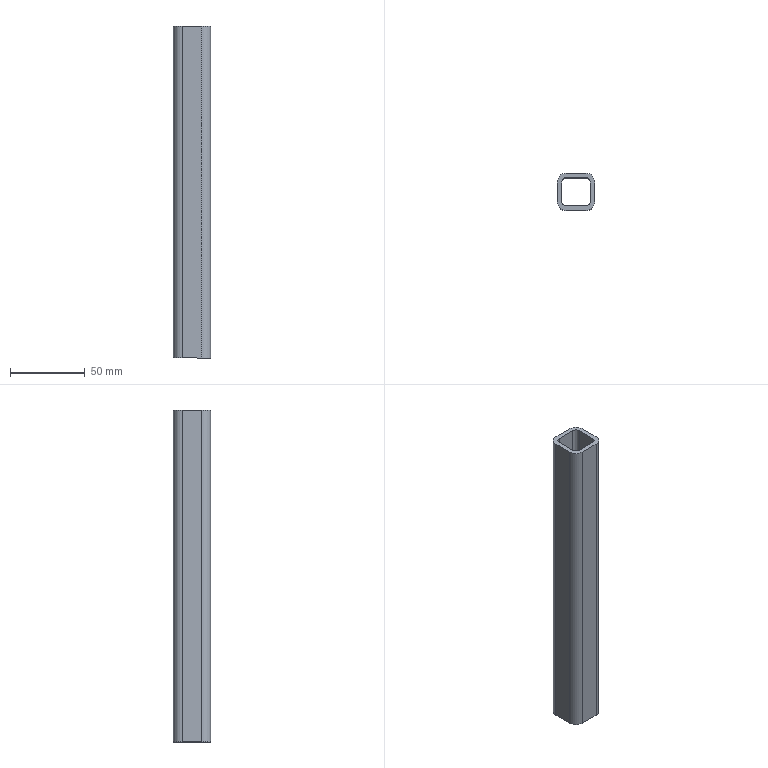Part | STEP file | ISO 10799-2 25x25x3 1784905468899 | 1 solid | 18 faces | box 25 x 25 x 222.2 mm | volume 53511 mm3 | plane 10 | cylinder 8 | commonest cylinder face diameters 6 x4 12 x4
STEP:
#1=CARTESIAN_POINT('',(-6.5,-9.5,247.2));
#2=VERTEX_POINT('',#1);
#3=CARTESIAN_POINT('',(6.5,-9.5,247.2));
#4=VERTEX_POINT('',#3);
#5=CARTESIAN_POINT('',(3.25,-9.5,247.2));
#6=DIRECTION('',(1.,0.,0.));
#7=VECTOR('',#6,10.);
#8=LINE('',#5,#7);
#9=EDGE_CURVE('',#2,#4,#8,.T.);
#10=ORIENTED_EDGE('',*,*,#9,.T.);
#11=CARTESIAN_POINT('',(6.5,-9.5,25.));
#12=VERTEX_POINT('',#11);
#13=CARTESIAN_POINT('',(6.5,-9.5,0.));
#14=DIRECTION('',(0.,0.,1.));
#15=VECTOR('',#14,10.);
#16=LINE('',#13,#15);
#17=EDGE_CURVE('',#12,#4,#16,.T.);
#18=ORIENTED_EDGE('',*,*,#17,.F.);
#19=CARTESIAN_POINT('',(-6.5,-9.5,25.));
#20=VERTEX_POINT('',#19);
#21=CARTESIAN_POINT('',(3.25,-9.5,25.));
#22=DIRECTION('',(1.,0.,0.));
#23=VECTOR('',#22,10.);
#24=LINE('',#21,#23);
#25=EDGE_CURVE('',#20,#12,#24,.T.);
#26=ORIENTED_EDGE('',*,*,#25,.F.);
#27=CARTESIAN_POINT('',(-6.5,-9.5,0.));
#28=DIRECTION('',(0.,0.,1.));
#29=VECTOR('',#28,10.);
#30=LINE('',#27,#29);
#31=EDGE_CURVE('',#20,#2,#30,.T.);
#32=ORIENTED_EDGE('',*,*,#31,.T.);
#33=EDGE_LOOP('',(#10,#18,#26,#32));
#34=FACE_OUTER_BOUND('',#33,.T.);
#35=CARTESIAN_POINT('',(6.5,-9.5,0.));
#36=DIRECTION('',(0.,-1.,0.));
#37=DIRECTION('',(0.,0.,-1.));
#38=AXIS2_PLACEMENT_3D('',#35,#36,#37);
#39=PLANE('',#38);
#40=ADVANCED_FACE('',(#34),#39,.F.);
#41=CARTESIAN_POINT('',(9.5,-6.5,247.2));
#42=VERTEX_POINT('',#41);
#43=CARTESIAN_POINT('',(6.5,-6.5,247.2));
#44=DIRECTION('',(0.,0.,1.));
#45=DIRECTION('',(0.,1.,0.));
#46=AXIS2_PLACEMENT_3D('',#43,#44,#45);
#47=CIRCLE('',#46,3.);
#48=EDGE_CURVE('',#4,#42,#47,.T.);
#49=ORIENTED_EDGE('',*,*,#48,.T.);
#50=CARTESIAN_POINT('',(9.5,-6.5,25.));
#51=VERTEX_POINT('',#50);
#52=CARTESIAN_POINT('',(9.5,-6.5,0.));
#53=DIRECTION('',(0.,0.,1.));
#54=VECTOR('',#53,10.);
#55=LINE('',#52,#54);
#56=EDGE_CURVE('',#51,#42,#55,.T.);
#57=ORIENTED_EDGE('',*,*,#56,.F.);
#58=CARTESIAN_POINT('',(6.5,-6.5,25.));
#59=DIRECTION('',(0.,0.,1.));
#60=DIRECTION('',(0.,1.,0.));
#61=AXIS2_PLACEMENT_3D('',#58,#59,#60);
#62=CIRCLE('',#61,3.);
#63=EDGE_CURVE('',#12,#51,#62,.T.);
#64=ORIENTED_EDGE('',*,*,#63,.F.);
#65=ORIENTED_EDGE('',*,*,#17,.T.);
#66=EDGE_LOOP('',(#49,#57,#64,#65));
#67=FACE_OUTER_BOUND('',#66,.T.);
#68=CARTESIAN_POINT('',(6.5,-6.5,0.));
#69=DIRECTION('',(0.,0.,1.));
#70=DIRECTION('',(0.,1.,0.));
#71=AXIS2_PLACEMENT_3D('',#68,#69,#70);
#72=CYLINDRICAL_SURFACE('',#71,3.);
#73=ADVANCED_FACE('',(#67),#72,.F.);
#74=CARTESIAN_POINT('',(9.5,6.5,247.2));
#75=VERTEX_POINT('',#74);
#76=CARTESIAN_POINT('',(9.5,3.25,247.2));
#77=DIRECTION('',(0.,1.,0.));
#78=VECTOR('',#77,10.);
#79=LINE('',#76,#78);
#80=EDGE_CURVE('',#42,#75,#79,.T.);
#81=ORIENTED_EDGE('',*,*,#80,.T.);
#82=CARTESIAN_POINT('',(9.5,6.5,25.));
#83=VERTEX_POINT('',#82);
#84=CARTESIAN_POINT('',(9.5,6.5,0.));
#85=DIRECTION('',(0.,0.,1.));
#86=VECTOR('',#85,10.);
#87=LINE('',#84,#86);
#88=EDGE_CURVE('',#83,#75,#87,.T.);
#89=ORIENTED_EDGE('',*,*,#88,.F.);
#90=CARTESIAN_POINT('',(9.5,3.25,25.));
#91=DIRECTION('',(0.,1.,0.));
#92=VECTOR('',#91,10.);
#93=LINE('',#90,#92);
#94=EDGE_CURVE('',#51,#83,#93,.T.);
#95=ORIENTED_EDGE('',*,*,#94,.F.);
#96=ORIENTED_EDGE('',*,*,#56,.T.);
#97=EDGE_LOOP('',(#81,#89,#95,#96));
#98=FACE_OUTER_BOUND('',#97,.T.);
#99=CARTESIAN_POINT('',(9.5,6.5,0.));
#100=DIRECTION('',(1.,0.,0.));
#101=DIRECTION('',(0.,0.,-1.));
#102=AXIS2_PLACEMENT_3D('',#99,#100,#101);
#103=PLANE('',#102);
#104=ADVANCED_FACE('',(#98),#103,.F.);
#105=CARTESIAN_POINT('',(6.5,9.5,247.2));
#106=VERTEX_POINT('',#105);
#107=CARTESIAN_POINT('',(6.5,6.5,247.2));
#108=DIRECTION('',(0.,0.,1.));
#109=DIRECTION('',(-1.,0.,0.));
#110=AXIS2_PLACEMENT_3D('',#107,#108,#109);
#111=CIRCLE('',#110,3.);
#112=EDGE_CURVE('',#75,#106,#111,.T.);
#113=ORIENTED_EDGE('',*,*,#112,.T.);
#114=CARTESIAN_POINT('',(6.5,9.5,25.));
#115=VERTEX_POINT('',#114);
#116=CARTESIAN_POINT('',(6.5,9.5,0.));
#117=DIRECTION('',(0.,0.,1.));
#118=VECTOR('',#117,10.);
#119=LINE('',#116,#118);
#120=EDGE_CURVE('',#115,#106,#119,.T.);
#121=ORIENTED_EDGE('',*,*,#120,.F.);
#122=CARTESIAN_POINT('',(6.5,6.5,25.));
#123=DIRECTION('',(0.,0.,1.));
#124=DIRECTION('',(-1.,0.,0.));
#125=AXIS2_PLACEMENT_3D('',#122,#123,#124);
#126=CIRCLE('',#125,3.);
#127=EDGE_CURVE('',#83,#115,#126,.T.);
#128=ORIENTED_EDGE('',*,*,#127,.F.);
#129=ORIENTED_EDGE('',*,*,#88,.T.);
#130=EDGE_LOOP('',(#113,#121,#128,#129));
#131=FACE_OUTER_BOUND('',#130,.T.);
#132=CARTESIAN_POINT('',(6.5,6.5,0.));
#133=DIRECTION('',(0.,0.,1.));
#134=DIRECTION('',(-1.,0.,0.));
#135=AXIS2_PLACEMENT_3D('',#132,#133,#134);
#136=CYLINDRICAL_SURFACE('',#135,3.);
#137=ADVANCED_FACE('',(#131),#136,.F.);
#138=CARTESIAN_POINT('',(12.5,6.5,247.2));
#139=VERTEX_POINT('',#138);
#140=CARTESIAN_POINT('',(12.5,-6.5,247.2));
#141=VERTEX_POINT('',#140);
#142=CARTESIAN_POINT('',(12.5,3.25,247.2));
#143=DIRECTION('',(0.,-1.,0.));
#144=VECTOR('',#143,10.);
#145=LINE('',#142,#144);
#146=EDGE_CURVE('',#139,#141,#145,.T.);
#147=ORIENTED_EDGE('',*,*,#146,.T.);
#148=CARTESIAN_POINT('',(12.5,-6.5,25.));
#149=VERTEX_POINT('',#148);
#150=CARTESIAN_POINT('',(12.5,-6.5,0.));
#151=DIRECTION('',(0.,0.,1.));
#152=VECTOR('',#151,10.);
#153=LINE('',#150,#152);
#154=EDGE_CURVE('',#149,#141,#153,.T.);
#155=ORIENTED_EDGE('',*,*,#154,.F.);
#156=CARTESIAN_POINT('',(12.5,6.5,25.));
#157=VERTEX_POINT('',#156);
#158=CARTESIAN_POINT('',(12.5,3.25,25.));
#159=DIRECTION('',(0.,-1.,0.));
#160=VECTOR('',#159,10.);
#161=LINE('',#158,#160);
#162=EDGE_CURVE('',#157,#149,#161,.T.);
#163=ORIENTED_EDGE('',*,*,#162,.F.);
#164=CARTESIAN_POINT('',(12.5,6.5,0.));
#165=DIRECTION('',(0.,0.,1.));
#166=VECTOR('',#165,10.);
#167=LINE('',#164,#166);
#168=EDGE_CURVE('',#157,#139,#167,.T.);
#169=ORIENTED_EDGE('',*,*,#168,.T.);
#170=EDGE_LOOP('',(#147,#155,#163,#169));
#171=FACE_OUTER_BOUND('',#170,.T.);
#172=CARTESIAN_POINT('',(12.5,6.5,0.));
#173=DIRECTION('',(1.,0.,0.));
#174=DIRECTION('',(0.,0.,-1.));
#175=AXIS2_PLACEMENT_3D('',#172,#173,#174);
#176=PLANE('',#175);
#177=ADVANCED_FACE('',(#171),#176,.T.);
#178=CARTESIAN_POINT('',(6.5,-12.5,247.2));
#179=VERTEX_POINT('',#178);
#180=CARTESIAN_POINT('',(6.5,-6.5,247.2));
#181=DIRECTION('',(0.,0.,-1.));
#182=DIRECTION('',(0.,1.,0.));
#183=AXIS2_PLACEMENT_3D('',#180,#181,#182);
#184=CIRCLE('',#183,6.);
#185=EDGE_CURVE('',#141,#179,#184,.T.);
#186=ORIENTED_EDGE('',*,*,#185,.T.);
#187=CARTESIAN_POINT('',(6.5,-12.5,25.));
#188=VERTEX_POINT('',#187);
#189=CARTESIAN_POINT('',(6.5,-12.5,0.));
#190=DIRECTION('',(0.,0.,1.));
#191=VECTOR('',#190,10.);
#192=LINE('',#189,#191);
#193=EDGE_CURVE('',#188,#179,#192,.T.);
#194=ORIENTED_EDGE('',*,*,#193,.F.);
#195=CARTESIAN_POINT('',(6.5,-6.5,25.));
#196=DIRECTION('',(0.,0.,-1.));
#197=DIRECTION('',(0.,1.,0.));
#198=AXIS2_PLACEMENT_3D('',#195,#196,#197);
#199=CIRCLE('',#198,6.);
#200=EDGE_CURVE('',#149,#188,#199,.T.);
#201=ORIENTED_EDGE('',*,*,#200,.F.);
#202=ORIENTED_EDGE('',*,*,#154,.T.);
#203=EDGE_LOOP('',(#186,#194,#201,#202));
#204=FACE_OUTER_BOUND('',#203,.T.);
#205=CARTESIAN_POINT('',(6.5,-6.5,0.));
#206=DIRECTION('',(0.,0.,1.));
#207=DIRECTION('',(0.,1.,0.));
#208=AXIS2_PLACEMENT_3D('',#205,#206,#207);
#209=CYLINDRICAL_SURFACE('',#208,6.);
#210=ADVANCED_FACE('',(#204),#209,.T.);
#211=CARTESIAN_POINT('',(-6.5,-12.5,247.2));
#212=VERTEX_POINT('',#211);
#213=CARTESIAN_POINT('',(3.25,-12.5,247.2));
#214=DIRECTION('',(-1.,0.,0.));
#215=VECTOR('',#214,10.);
#216=LINE('',#213,#215);
#217=EDGE_CURVE('',#179,#212,#216,.T.);
#218=ORIENTED_EDGE('',*,*,#217,.T.);
#219=CARTESIAN_POINT('',(-6.5,-12.5,25.));
#220=VERTEX_POINT('',#219);
#221=CARTESIAN_POINT('',(-6.5,-12.5,0.));
#222=DIRECTION('',(0.,0.,1.));
#223=VECTOR('',#222,10.);
#224=LINE('',#221,#223);
#225=EDGE_CURVE('',#220,#212,#224,.T.);
#226=ORIENTED_EDGE('',*,*,#225,.F.);
#227=CARTESIAN_POINT('',(3.25,-12.5,25.));
#228=DIRECTION('',(-1.,0.,0.));
#229=VECTOR('',#228,10.);
#230=LINE('',#227,#229);
#231=EDGE_CURVE('',#188,#220,#230,.T.);
#232=ORIENTED_EDGE('',*,*,#231,.F.);
#233=ORIENTED_EDGE('',*,*,#193,.T.);
#234=EDGE_LOOP('',(#218,#226,#232,#233));
#235=FACE_OUTER_BOUND('',#234,.T.);
#236=CARTESIAN_POINT('',(6.5,-12.5,0.));
#237=DIRECTION('',(0.,-1.,0.));
#238=DIRECTION('',(0.,0.,-1.));
#239=AXIS2_PLACEMENT_3D('',#236,#237,#238);
#240=PLANE('',#239);
#241=ADVANCED_FACE('',(#235),#240,.T.);
#242=CARTESIAN_POINT('',(-12.5,-6.5,247.2));
#243=VERTEX_POINT('',#242);
#244=CARTESIAN_POINT('',(-6.5,-6.5,247.2));
#245=DIRECTION('',(0.,0.,-1.));
#246=DIRECTION('',(1.,0.,0.));
#247=AXIS2_PLACEMENT_3D('',#244,#245,#246);
#248=CIRCLE('',#247,6.);
#249=EDGE_CURVE('',#212,#243,#248,.T.);
#250=ORIENTED_EDGE('',*,*,#249,.T.);
#251=CARTESIAN_POINT('',(-12.5,-6.5,25.));
#252=VERTEX_POINT('',#251);
#253=CARTESIAN_POINT('',(-12.5,-6.5,0.));
#254=DIRECTION('',(0.,0.,1.));
#255=VECTOR('',#254,10.);
#256=LINE('',#253,#255);
#257=EDGE_CURVE('',#252,#243,#256,.T.);
#258=ORIENTED_EDGE('',*,*,#257,.F.);
#259=CARTESIAN_POINT('',(-6.5,-6.5,25.));
#260=DIRECTION('',(0.,0.,-1.));
#261=DIRECTION('',(1.,0.,0.));
#262=AXIS2_PLACEMENT_3D('',#259,#260,#261);
#263=CIRCLE('',#262,6.);
#264=EDGE_CURVE('',#220,#252,#263,.T.);
#265=ORIENTED_EDGE('',*,*,#264,.F.);
#266=ORIENTED_EDGE('',*,*,#225,.T.);
#267=EDGE_LOOP('',(#250,#258,#265,#266));
#268=FACE_OUTER_BOUND('',#267,.T.);
#269=CARTESIAN_POINT('',(-6.5,-6.5,0.));
#270=DIRECTION('',(0.,0.,1.));
#271=DIRECTION('',(1.,0.,0.));
#272=AXIS2_PLACEMENT_3D('',#269,#270,#271);
#273=CYLINDRICAL_SURFACE('',#272,6.);
#274=ADVANCED_FACE('',(#268),#273,.T.);
#275=CARTESIAN_POINT('',(-6.5,9.5,247.2));
#276=VERTEX_POINT('',#275);
#277=CARTESIAN_POINT('',(-3.25,9.5,247.2));
#278=DIRECTION('',(-1.,0.,0.));
#279=VECTOR('',#278,10.);
#280=LINE('',#277,#279);
#281=EDGE_CURVE('',#106,#276,#280,.T.);
#282=ORIENTED_EDGE('',*,*,#281,.T.);
#283=CARTESIAN_POINT('',(-6.5,9.5,25.));
#284=VERTEX_POINT('',#283);
#285=CARTESIAN_POINT('',(-6.5,9.5,0.));
#286=DIRECTION('',(0.,0.,1.));
#287=VECTOR('',#286,10.);
#288=LINE('',#285,#287);
#289=EDGE_CURVE('',#284,#276,#288,.T.);
#290=ORIENTED_EDGE('',*,*,#289,.F.);
#291=CARTESIAN_POINT('',(-3.25,9.5,25.));
#292=DIRECTION('',(-1.,0.,0.));
#293=VECTOR('',#292,10.);
#294=LINE('',#291,#293);
#295=EDGE_CURVE('',#115,#284,#294,.T.);
#296=ORIENTED_EDGE('',*,*,#295,.F.);
#297=ORIENTED_EDGE('',*,*,#120,.T.);
#298=EDGE_LOOP('',(#282,#290,#296,#297));
#299=FACE_OUTER_BOUND('',#298,.T.);
#300=CARTESIAN_POINT('',(-6.5,9.5,0.));
#301=DIRECTION('',(0.,1.,0.));
#302=DIRECTION('',(0.,0.,1.));
#303=AXIS2_PLACEMENT_3D('',#300,#301,#302);
#304=PLANE('',#303);
#305=ADVANCED_FACE('',(#299),#304,.F.);
#306=CARTESIAN_POINT('',(-9.5,-6.5,247.2));
#307=VERTEX_POINT('',#306);
#308=CARTESIAN_POINT('',(-6.5,-6.5,247.2));
#309=DIRECTION('',(0.,0.,1.));
#310=DIRECTION('',(1.,0.,0.));
#311=AXIS2_PLACEMENT_3D('',#308,#309,#310);
#312=CIRCLE('',#311,3.);
#313=EDGE_CURVE('',#307,#2,#312,.T.);
#314=ORIENTED_EDGE('',*,*,#313,.T.);
#315=ORIENTED_EDGE('',*,*,#31,.F.);
#316=CARTESIAN_POINT('',(-9.5,-6.5,25.));
#317=VERTEX_POINT('',#316);
#318=CARTESIAN_POINT('',(-6.5,-6.5,25.));
#319=DIRECTION('',(0.,0.,1.));
#320=DIRECTION('',(1.,0.,0.));
#321=AXIS2_PLACEMENT_3D('',#318,#319,#320);
#322=CIRCLE('',#321,3.);
#323=EDGE_CURVE('',#317,#20,#322,.T.);
#324=ORIENTED_EDGE('',*,*,#323,.F.);
#325=CARTESIAN_POINT('',(-9.5,-6.5,0.));
#326=DIRECTION('',(0.,0.,1.));
#327=VECTOR('',#326,10.);
#328=LINE('',#325,#327);
#329=EDGE_CURVE('',#317,#307,#328,.T.);
#330=ORIENTED_EDGE('',*,*,#329,.T.);
#331=EDGE_LOOP('',(#314,#315,#324,#330));
#332=FACE_OUTER_BOUND('',#331,.T.);
#333=CARTESIAN_POINT('',(-6.5,-6.5,0.));
#334=DIRECTION('',(0.,0.,1.));
#335=DIRECTION('',(1.,0.,0.));
#336=AXIS2_PLACEMENT_3D('',#333,#334,#335);
#337=CYLINDRICAL_SURFACE('',#336,3.);
#338=ADVANCED_FACE('',(#332),#337,.F.);
#339=CARTESIAN_POINT('',(-9.5,6.5,247.2));
#340=VERTEX_POINT('',#339);
#341=CARTESIAN_POINT('',(-9.5,-3.25,247.2));
#342=DIRECTION('',(0.,-1.,0.));
#343=VECTOR('',#342,10.);
#344=LINE('',#341,#343);
#345=EDGE_CURVE('',#340,#307,#344,.T.);
#346=ORIENTED_EDGE('',*,*,#345,.T.);
#347=ORIENTED_EDGE('',*,*,#329,.F.);
#348=CARTESIAN_POINT('',(-9.5,6.5,25.));
#349=VERTEX_POINT('',#348);
#350=CARTESIAN_POINT('',(-9.5,-3.25,25.));
#351=DIRECTION('',(0.,-1.,0.));
#352=VECTOR('',#351,10.);
#353=LINE('',#350,#352);
#354=EDGE_CURVE('',#349,#317,#353,.T.);
#355=ORIENTED_EDGE('',*,*,#354,.F.);
#356=CARTESIAN_POINT('',(-9.5,6.5,0.));
#357=DIRECTION('',(0.,0.,1.));
#358=VECTOR('',#357,10.);
#359=LINE('',#356,#358);
#360=EDGE_CURVE('',#349,#340,#359,.T.);
#361=ORIENTED_EDGE('',*,*,#360,.T.);
#362=EDGE_LOOP('',(#346,#347,#355,#361));
#363=FACE_OUTER_BOUND('',#362,.T.);
#364=CARTESIAN_POINT('',(-9.5,-6.5,0.));
#365=DIRECTION('',(-1.,0.,0.));
#366=DIRECTION('',(0.,0.,1.));
#367=AXIS2_PLACEMENT_3D('',#364,#365,#366);
#368=PLANE('',#367);
#369=ADVANCED_FACE('',(#363),#368,.F.);
#370=CARTESIAN_POINT('',(-6.5,6.5,247.2));
#371=DIRECTION('',(0.,0.,1.));
#372=DIRECTION('',(0.,-1.,0.));
#373=AXIS2_PLACEMENT_3D('',#370,#371,#372);
#374=CIRCLE('',#373,3.);
#375=EDGE_CURVE('',#276,#340,#374,.T.);
#376=ORIENTED_EDGE('',*,*,#375,.T.);
#377=ORIENTED_EDGE('',*,*,#360,.F.);
#378=CARTESIAN_POINT('',(-6.5,6.5,25.));
#379=DIRECTION('',(0.,0.,1.));
#380=DIRECTION('',(0.,-1.,0.));
#381=AXIS2_PLACEMENT_3D('',#378,#379,#380);
#382=CIRCLE('',#381,3.);
#383=EDGE_CURVE('',#284,#349,#382,.T.);
#384=ORIENTED_EDGE('',*,*,#383,.F.);
#385=ORIENTED_EDGE('',*,*,#289,.T.);
#386=EDGE_LOOP('',(#376,#377,#384,#385));
#387=FACE_OUTER_BOUND('',#386,.T.);
#388=CARTESIAN_POINT('',(-6.5,6.5,0.));
#389=DIRECTION('',(0.,0.,1.));
#390=DIRECTION('',(0.,-1.,0.));
#391=AXIS2_PLACEMENT_3D('',#388,#389,#390);
#392=CYLINDRICAL_SURFACE('',#391,3.);
#393=ADVANCED_FACE('',(#387),#392,.F.);
#394=CARTESIAN_POINT('',(-12.5,6.5,247.2));
#395=VERTEX_POINT('',#394);
#396=CARTESIAN_POINT('',(-12.5,-3.25,247.2));
#397=DIRECTION('',(0.,1.,0.));
#398=VECTOR('',#397,10.);
#399=LINE('',#396,#398);
#400=EDGE_CURVE('',#243,#395,#399,.T.);
#401=ORIENTED_EDGE('',*,*,#400,.T.);
#402=CARTESIAN_POINT('',(-12.5,6.5,25.));
#403=VERTEX_POINT('',#402);
#404=CARTESIAN_POINT('',(-12.5,6.5,0.));
#405=DIRECTION('',(0.,0.,1.));
#406=VECTOR('',#405,10.);
#407=LINE('',#404,#406);
#408=EDGE_CURVE('',#403,#395,#407,.T.);
#409=ORIENTED_EDGE('',*,*,#408,.F.);
#410=CARTESIAN_POINT('',(-12.5,-3.25,25.));
#411=DIRECTION('',(0.,1.,0.));
#412=VECTOR('',#411,10.);
#413=LINE('',#410,#412);
#414=EDGE_CURVE('',#252,#403,#413,.T.);
#415=ORIENTED_EDGE('',*,*,#414,.F.);
#416=ORIENTED_EDGE('',*,*,#257,.T.);
#417=EDGE_LOOP('',(#401,#409,#415,#416));
#418=FACE_OUTER_BOUND('',#417,.T.);
#419=CARTESIAN_POINT('',(-12.5,-6.5,0.));
#420=DIRECTION('',(-1.,0.,0.));
#421=DIRECTION('',(0.,0.,1.));
#422=AXIS2_PLACEMENT_3D('',#419,#420,#421);
#423=PLANE('',#422);
#424=ADVANCED_FACE('',(#418),#423,.T.);
#425=CARTESIAN_POINT('',(-6.5,12.5,247.2));
#426=VERTEX_POINT('',#425);
#427=CARTESIAN_POINT('',(-6.5,6.5,247.2));
#428=DIRECTION('',(0.,0.,-1.));
#429=DIRECTION('',(0.,-1.,0.));
#430=AXIS2_PLACEMENT_3D('',#427,#428,#429);
#431=CIRCLE('',#430,6.);
#432=EDGE_CURVE('',#395,#426,#431,.T.);
#433=ORIENTED_EDGE('',*,*,#432,.T.);
#434=CARTESIAN_POINT('',(-6.5,12.5,25.));
#435=VERTEX_POINT('',#434);
#436=CARTESIAN_POINT('',(-6.5,12.5,0.));
#437=DIRECTION('',(0.,0.,1.));
#438=VECTOR('',#437,10.);
#439=LINE('',#436,#438);
#440=EDGE_CURVE('',#435,#426,#439,.T.);
#441=ORIENTED_EDGE('',*,*,#440,.F.);
#442=CARTESIAN_POINT('',(-6.5,6.5,25.));
#443=DIRECTION('',(0.,0.,-1.));
#444=DIRECTION('',(0.,-1.,0.));
#445=AXIS2_PLACEMENT_3D('',#442,#443,#444);
#446=CIRCLE('',#445,6.);
#447=EDGE_CURVE('',#403,#435,#446,.T.);
#448=ORIENTED_EDGE('',*,*,#447,.F.);
#449=ORIENTED_EDGE('',*,*,#408,.T.);
#450=EDGE_LOOP('',(#433,#441,#448,#449));
#451=FACE_OUTER_BOUND('',#450,.T.);
#452=CARTESIAN_POINT('',(-6.5,6.5,0.));
#453=DIRECTION('',(0.,0.,1.));
#454=DIRECTION('',(0.,-1.,0.));
#455=AXIS2_PLACEMENT_3D('',#452,#453,#454);
#456=CYLINDRICAL_SURFACE('',#455,6.);
#457=ADVANCED_FACE('',(#451),#456,.T.);
#458=CARTESIAN_POINT('',(6.5,12.5,247.2));
#459=VERTEX_POINT('',#458);
#460=CARTESIAN_POINT('',(-3.25,12.5,247.2));
#461=DIRECTION('',(1.,0.,0.));
#462=VECTOR('',#461,10.);
#463=LINE('',#460,#462);
#464=EDGE_CURVE('',#426,#459,#463,.T.);
#465=ORIENTED_EDGE('',*,*,#464,.T.);
#466=CARTESIAN_POINT('',(6.5,12.5,25.));
#467=VERTEX_POINT('',#466);
#468=CARTESIAN_POINT('',(6.5,12.5,0.));
#469=DIRECTION('',(0.,0.,1.));
#470=VECTOR('',#469,10.);
#471=LINE('',#468,#470);
#472=EDGE_CURVE('',#467,#459,#471,.T.);
#473=ORIENTED_EDGE('',*,*,#472,.F.);
#474=CARTESIAN_POINT('',(-3.25,12.5,25.));
#475=DIRECTION('',(1.,0.,0.));
#476=VECTOR('',#475,10.);
#477=LINE('',#474,#476);
#478=EDGE_CURVE('',#435,#467,#477,.T.);
#479=ORIENTED_EDGE('',*,*,#478,.F.);
#480=ORIENTED_EDGE('',*,*,#440,.T.);
#481=EDGE_LOOP('',(#465,#473,#479,#480));
#482=FACE_OUTER_BOUND('',#481,.T.);
#483=CARTESIAN_POINT('',(-6.5,12.5,0.));
#484=DIRECTION('',(0.,1.,0.));
#485=DIRECTION('',(0.,0.,1.));
#486=AXIS2_PLACEMENT_3D('',#483,#484,#485);
#487=PLANE('',#486);
#488=ADVANCED_FACE('',(#482),#487,.T.);
#489=CARTESIAN_POINT('',(6.5,6.5,247.2));
#490=DIRECTION('',(0.,0.,-1.));
#491=DIRECTION('',(-1.,0.,0.));
#492=AXIS2_PLACEMENT_3D('',#489,#490,#491);
#493=CIRCLE('',#492,6.);
#494=EDGE_CURVE('',#459,#139,#493,.T.);
#495=ORIENTED_EDGE('',*,*,#494,.T.);
#496=ORIENTED_EDGE('',*,*,#168,.F.);
#497=CARTESIAN_POINT('',(6.5,6.5,25.));
#498=DIRECTION('',(0.,0.,-1.));
#499=DIRECTION('',(-1.,0.,0.));
#500=AXIS2_PLACEMENT_3D('',#497,#498,#499);
#501=CIRCLE('',#500,6.);
#502=EDGE_CURVE('',#467,#157,#501,.T.);
#503=ORIENTED_EDGE('',*,*,#502,.F.);
#504=ORIENTED_EDGE('',*,*,#472,.T.);
#505=EDGE_LOOP('',(#495,#496,#503,#504));
#506=FACE_OUTER_BOUND('',#505,.T.);
#507=CARTESIAN_POINT('',(6.5,6.5,0.));
#508=DIRECTION('',(0.,0.,1.));
#509=DIRECTION('',(-1.,0.,0.));
#510=AXIS2_PLACEMENT_3D('',#507,#508,#509);
#511=CYLINDRICAL_SURFACE('',#510,6.);
#512=ADVANCED_FACE('',(#506),#511,.T.);
#513=ORIENTED_EDGE('',*,*,#414,.T.);
#514=ORIENTED_EDGE('',*,*,#447,.T.);
#515=ORIENTED_EDGE('',*,*,#478,.T.);
#516=ORIENTED_EDGE('',*,*,#502,.T.);
#517=ORIENTED_EDGE('',*,*,#162,.T.);
#518=ORIENTED_EDGE('',*,*,#200,.T.);
#519=ORIENTED_EDGE('',*,*,#231,.T.);
#520=ORIENTED_EDGE('',*,*,#264,.T.);
#521=EDGE_LOOP('',(#513,#514,#515,#516,#517,#518,#519,#520));
#522=FACE_OUTER_BOUND('',#521,.T.);
#523=ORIENTED_EDGE('',*,*,#295,.T.);
#524=ORIENTED_EDGE('',*,*,#383,.T.);
#525=ORIENTED_EDGE('',*,*,#354,.T.);
#526=ORIENTED_EDGE('',*,*,#323,.T.);
#527=ORIENTED_EDGE('',*,*,#25,.T.);
#528=ORIENTED_EDGE('',*,*,#63,.T.);
#529=ORIENTED_EDGE('',*,*,#94,.T.);
#530=ORIENTED_EDGE('',*,*,#127,.T.);
#531=EDGE_LOOP('',(#523,#524,#525,#526,#527,#528,#529,#530));
#532=FACE_BOUND('',#531,.T.);
#533=CARTESIAN_POINT('',(0.,0.,25.));
#534=DIRECTION('',(0.,0.,1.));
#535=DIRECTION('',(1.,0.,0.));
#536=AXIS2_PLACEMENT_3D('',#533,#534,#535);
#537=PLANE('',#536);
#538=ADVANCED_FACE('',(#522,#532),#537,.F.);
#539=ORIENTED_EDGE('',*,*,#400,.F.);
#540=ORIENTED_EDGE('',*,*,#249,.F.);
#541=ORIENTED_EDGE('',*,*,#217,.F.);
#542=ORIENTED_EDGE('',*,*,#185,.F.);
#543=ORIENTED_EDGE('',*,*,#146,.F.);
#544=ORIENTED_EDGE('',*,*,#494,.F.);
#545=ORIENTED_EDGE('',*,*,#464,.F.);
#546=ORIENTED_EDGE('',*,*,#432,.F.);
#547=EDGE_LOOP('',(#539,#540,#541,#542,#543,#544,#545,#546));
#548=FACE_OUTER_BOUND('',#547,.T.);
#549=ORIENTED_EDGE('',*,*,#281,.F.);
#550=ORIENTED_EDGE('',*,*,#112,.F.);
#551=ORIENTED_EDGE('',*,*,#80,.F.);
#552=ORIENTED_EDGE('',*,*,#48,.F.);
#553=ORIENTED_EDGE('',*,*,#9,.F.);
#554=ORIENTED_EDGE('',*,*,#313,.F.);
#555=ORIENTED_EDGE('',*,*,#345,.F.);
#556=ORIENTED_EDGE('',*,*,#375,.F.);
#557=EDGE_LOOP('',(#549,#550,#551,#552,#553,#554,#555,#556));
#558=FACE_BOUND('',#557,.T.);
#559=CARTESIAN_POINT('',(0.,0.,247.2));
#560=DIRECTION('',(0.,0.,1.));
#561=DIRECTION('',(1.,0.,0.));
#562=AXIS2_PLACEMENT_3D('',#559,#560,#561);
#563=PLANE('',#562);
#564=ADVANCED_FACE('',(#548,#558),#563,.T.);
#565=CLOSED_SHELL('',(#40,#73,#104,#137,#177,#210,#241,#274,#305,#338,#369,#393,#424,#457,#488,#512,#538,#564));
#566=MANIFOLD_SOLID_BREP('',#565);
#567=(LENGTH_UNIT()NAMED_UNIT(*)SI_UNIT(.MILLI.,.METRE.));
#568=UNCERTAINTY_MEASURE_WITH_UNIT(LENGTH_MEASURE(0.01),#567,'','');
#569=(NAMED_UNIT(*)PLANE_ANGLE_UNIT()SI_UNIT($,.RADIAN.));
#570=(NAMED_UNIT(*)SI_UNIT($,.STERADIAN.)SOLID_ANGLE_UNIT());
#571=(GEOMETRIC_REPRESENTATION_CONTEXT(3)GLOBAL_UNCERTAINTY_ASSIGNED_CONTEXT((#568))GLOBAL_UNIT_ASSIGNED_CONTEXT((#567,#569,#570))REPRESENTATION_CONTEXT('',''));
#572=ADVANCED_BREP_SHAPE_REPRESENTATION('',(#566),#571);